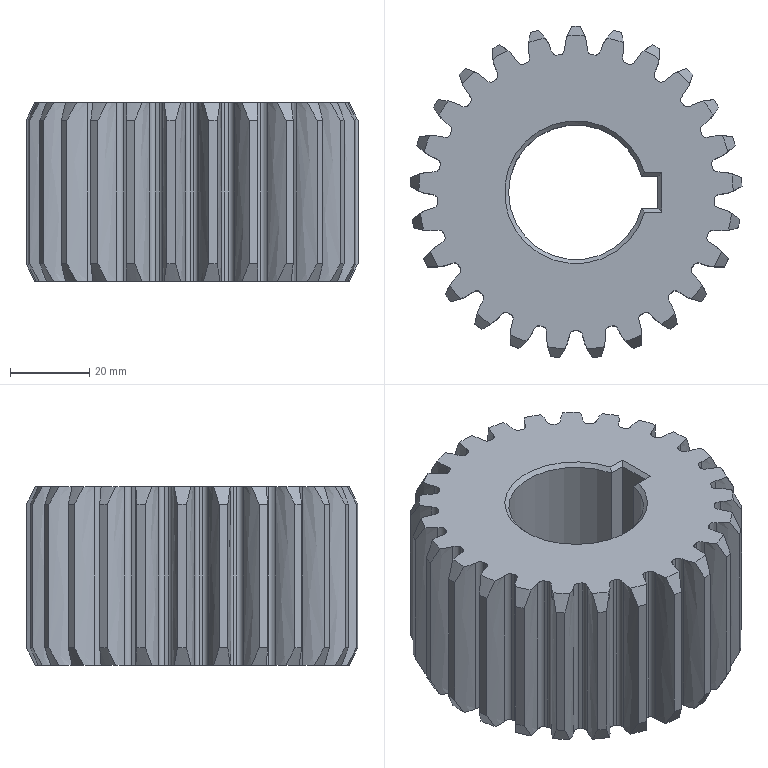Part | NX | features BREP 25, META 25, DATUM_CSYS 4, SKETCH 3, EXTRUDE 2, CHAMFER 1, CPROJ 1, CYLINDER 1, FSET 1, SWP104 1 | 1 solid | 214 faces | box 83.645 x 83.495 x 45 mm | volume 166384 mm3 | spline 125 | cone 52 | cylinder 26 | plane 11 | commonest cylinder face diameters 69.75 x25 34 x1